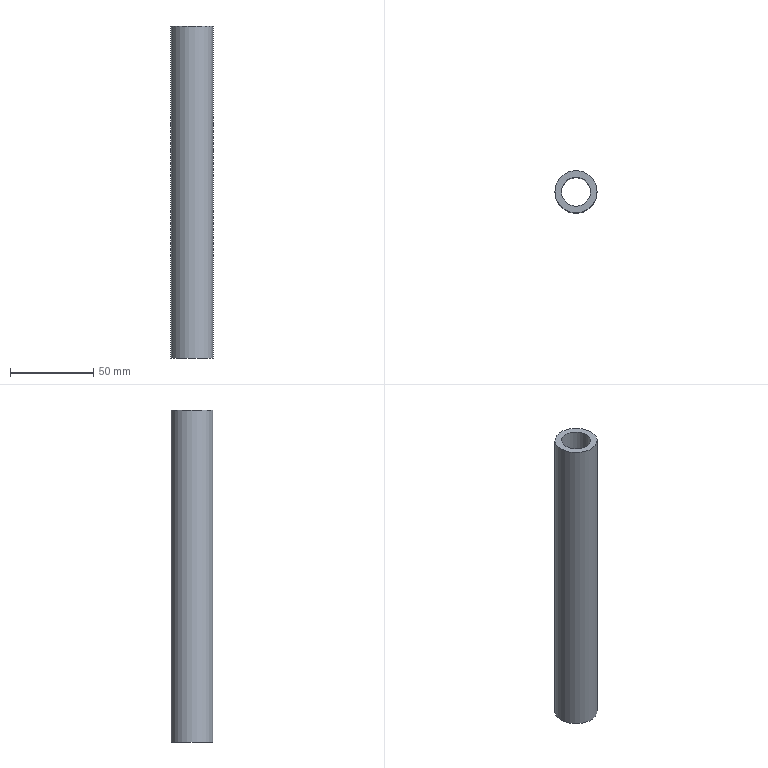Part | NX | features solid 2 | 1 solid | 4 faces | box 25.4 x 25.4 x 200 mm | volume 53784 mm3 | plane 2 | cylinder 2 | commonest cylinder face diameters 17.4 x1 25.4 x1
STEP:
#1=CARTESIAN_POINT('',(-236.3,370.,330.));
#2=VERTEX_POINT('',#1);
#3=CARTESIAN_POINT('',(-245.,370.,330.));
#4=DIRECTION('',(0.,0.,1.));
#5=DIRECTION('',(1.,0.,0.));
#6=AXIS2_PLACEMENT_3D('',#3,#4,#5);
#7=CIRCLE('',#6,8.7);
#8=EDGE_CURVE('',#2,#2,#7,.T.);
#9=ORIENTED_EDGE('',*,*,#8,.F.);
#10=EDGE_LOOP('',(#9));
#11=FACE_BOUND('',#10,.T.);
#12=CARTESIAN_POINT('',(-257.7,370.,330.));
#13=VERTEX_POINT('',#12);
#14=CARTESIAN_POINT('',(-245.,370.,330.));
#15=DIRECTION('',(0.,0.,1.));
#16=DIRECTION('',(-1.,0.,0.));
#17=AXIS2_PLACEMENT_3D('',#14,#15,#16);
#18=CIRCLE('',#17,12.7);
#19=EDGE_CURVE('',#13,#13,#18,.T.);
#20=ORIENTED_EDGE('',*,*,#19,.T.);
#21=EDGE_LOOP('',(#20));
#22=FACE_BOUND('',#21,.T.);
#23=CARTESIAN_POINT('',(-245.,370.,330.));
#24=DIRECTION('',(0.,0.,-1.));
#25=DIRECTION('',(-1.,0.,0.));
#26=AXIS2_PLACEMENT_3D('',#23,#24,#25);
#27=PLANE('',#26);
#28=ADVANCED_FACE('',(#11,#22),#27,.F.);
#29=CARTESIAN_POINT('',(-236.3,370.,130.));
#30=VERTEX_POINT('',#29);
#31=CARTESIAN_POINT('',(-245.,370.,130.));
#32=DIRECTION('',(0.,0.,1.));
#33=DIRECTION('',(1.,0.,0.));
#34=AXIS2_PLACEMENT_3D('',#31,#32,#33);
#35=CIRCLE('',#34,8.7);
#36=EDGE_CURVE('',#30,#30,#35,.T.);
#37=ORIENTED_EDGE('',*,*,#36,.T.);
#38=EDGE_LOOP('',(#37));
#39=FACE_BOUND('',#38,.T.);
#40=CARTESIAN_POINT('',(-257.7,370.,130.));
#41=VERTEX_POINT('',#40);
#42=CARTESIAN_POINT('',(-245.,370.,130.));
#43=DIRECTION('',(0.,0.,1.));
#44=DIRECTION('',(-1.,0.,0.));
#45=AXIS2_PLACEMENT_3D('',#42,#43,#44);
#46=CIRCLE('',#45,12.7);
#47=EDGE_CURVE('',#41,#41,#46,.T.);
#48=ORIENTED_EDGE('',*,*,#47,.F.);
#49=EDGE_LOOP('',(#48));
#50=FACE_BOUND('',#49,.T.);
#51=CARTESIAN_POINT('',(-245.,370.,130.));
#52=DIRECTION('',(0.,0.,-1.));
#53=DIRECTION('',(-1.,0.,0.));
#54=AXIS2_PLACEMENT_3D('',#51,#52,#53);
#55=PLANE('',#54);
#56=ADVANCED_FACE('',(#39,#50),#55,.T.);
#57=ORIENTED_EDGE('',*,*,#8,.T.);
#58=EDGE_LOOP('',(#57));
#59=FACE_BOUND('',#58,.T.);
#60=ORIENTED_EDGE('',*,*,#36,.F.);
#61=EDGE_LOOP('',(#60));
#62=FACE_BOUND('',#61,.T.);
#63=CARTESIAN_POINT('',(-245.,370.,130.));
#64=DIRECTION('',(0.,0.,1.));
#65=DIRECTION('',(1.,0.,0.));
#66=AXIS2_PLACEMENT_3D('',#63,#64,#65);
#67=CYLINDRICAL_SURFACE('',#66,8.7);
#68=ADVANCED_FACE('',(#59,#62),#67,.F.);
#69=ORIENTED_EDGE('',*,*,#19,.F.);
#70=EDGE_LOOP('',(#69));
#71=FACE_BOUND('',#70,.T.);
#72=ORIENTED_EDGE('',*,*,#47,.T.);
#73=EDGE_LOOP('',(#72));
#74=FACE_BOUND('',#73,.T.);
#75=CARTESIAN_POINT('',(-245.,370.,130.));
#76=DIRECTION('',(0.,0.,1.));
#77=DIRECTION('',(1.,0.,0.));
#78=AXIS2_PLACEMENT_3D('',#75,#76,#77);
#79=CYLINDRICAL_SURFACE('',#78,12.7);
#80=ADVANCED_FACE('',(#71,#74),#79,.T.);
#81=CLOSED_SHELL('',(#28,#56,#68,#80));
#82=MANIFOLD_SOLID_BREP('',#81);
#83=(LENGTH_UNIT()NAMED_UNIT(*)SI_UNIT(.MILLI.,.METRE.));
#84=UNCERTAINTY_MEASURE_WITH_UNIT(LENGTH_MEASURE(0.00001),#83,'','');
#85=(NAMED_UNIT(*)PLANE_ANGLE_UNIT()SI_UNIT($,.RADIAN.));
#86=(NAMED_UNIT(*)SI_UNIT($,.STERADIAN.)SOLID_ANGLE_UNIT());
#87=(GEOMETRIC_REPRESENTATION_CONTEXT(3)GLOBAL_UNCERTAINTY_ASSIGNED_CONTEXT((#84))GLOBAL_UNIT_ASSIGNED_CONTEXT((#83,#85,#86))REPRESENTATION_CONTEXT('',''));
#88=ADVANCED_BREP_SHAPE_REPRESENTATION('',(#82),#87);